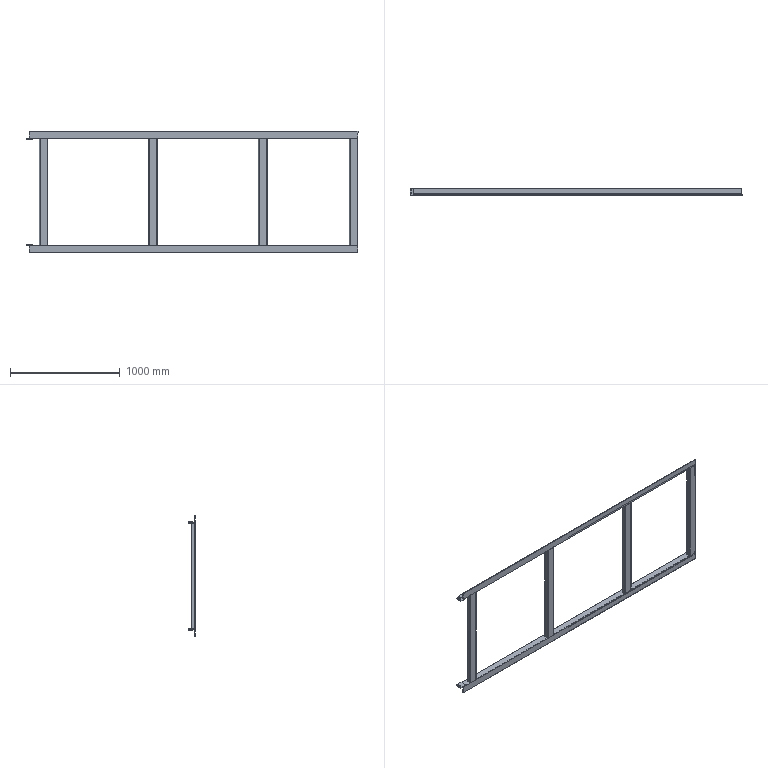Part | SolidWorks | features ICE 4, WeldMemberFeat 3, 3DProfileFeature 1, HoleWzd 1, LPattern 1, WeldmentFeature 1 | 8 solids | 114 faces | box 3030 x 63 x 1106 mm | volume 7792453 mm3 | plane 68 | cylinder 46 | commonest cylinder face diameters 8 x16 16 x16 10 x8 4 x4 14 x2